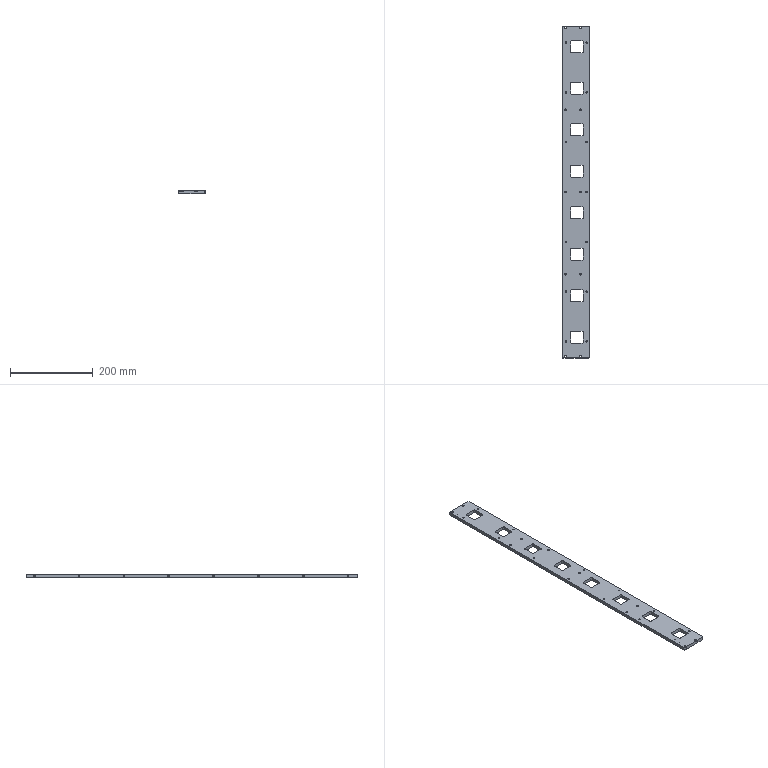Part | STEP file | SynoNew-0304-028 | 1 solid | 136 faces | box 65 x 800 x 8 mm | volume 354237 mm3 | cylinder 78 | plane 50 | cone 8 | commonest cylinder face diameters 6 x32 3.2 x14 8 x14 4.5 x10 4.2 x8